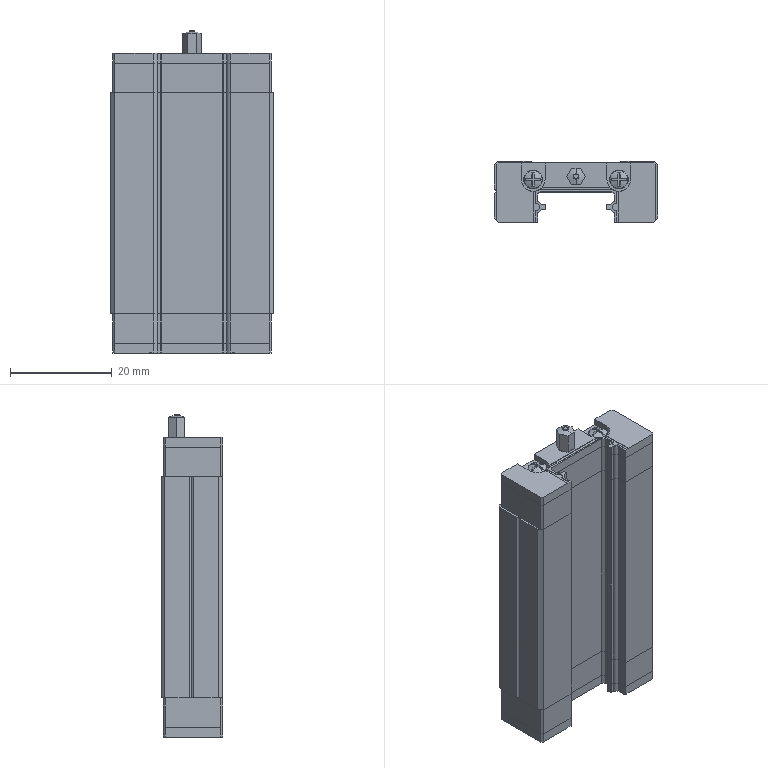Part | SolidWorks | features ICE 21, MirrorSolid 4, Extrusion 3, Fillet 3, MirrorPattern 3, RevCut 3, Chamfer 2, Dome 2, DeleteBody 1, LPattern 1, LibraryFeature 1 | 7 solids | 343 faces | box 32 x 12 x 63.373 mm | volume 16736 mm3 | plane 233 | cylinder 82 | torus 10 | cone 10 | sphere 8 | commonest cylinder face diameters 0.3 x20 2.372 x20 3 x12 2.4 x8 3.725 x8 1.444 x6